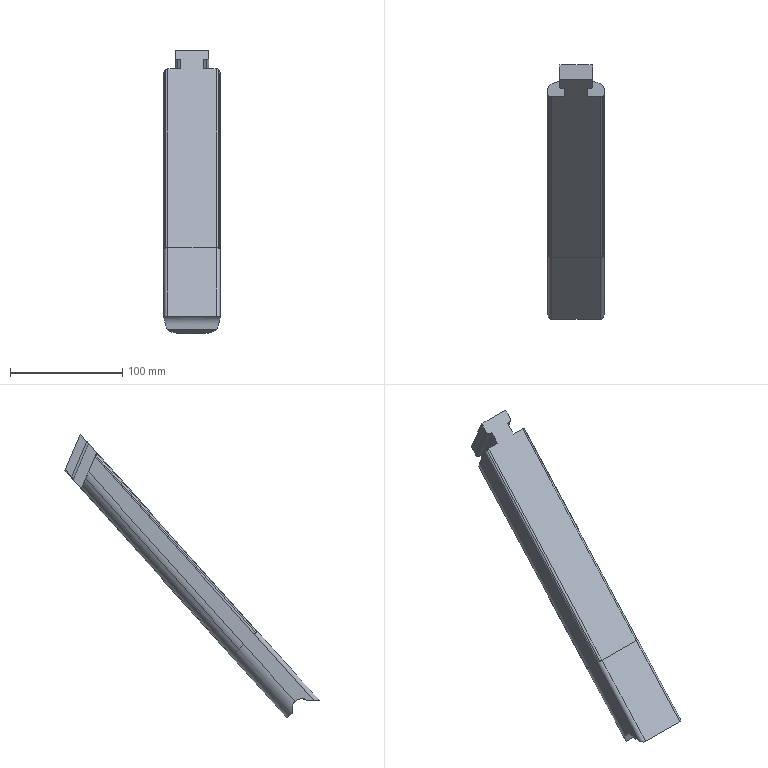Part | Creo | 1 solid | 37 faces | box 49.932 x 226.707 x 252.385 mm | volume 434284 mm3 | cylinder 19 | plane 17 | spline 1 | commonest cylinder face diameters 4 x2 7.029 x2 30.125 x2 30.2 x2 7.097 x1 7.12 x1